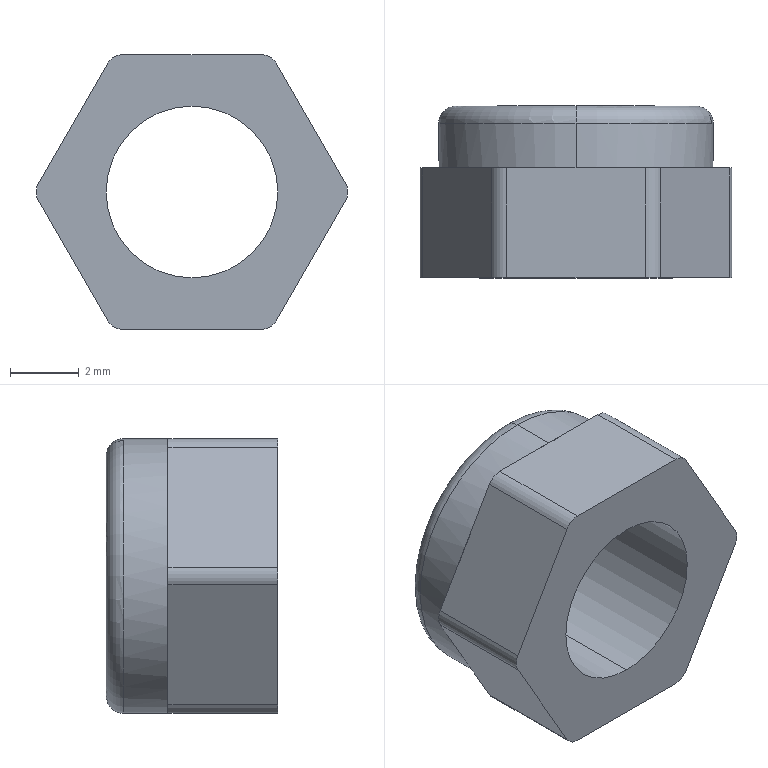Part | SolidWorks | features Extrusion 1, Fillet 1, ICE 1 | 1 solid | 28 faces | box 9.083 x 5 x 8 mm | volume 167.216 mm3 | plane 14 | cylinder 10 | torus 4 | commonest cylinder face diameters 1 x6 5 x2 8 x2
STEP:
#1=CARTESIAN_POINT('',(0.,4.5,-4.));
#2=VERTEX_POINT('',#1);
#3=CARTESIAN_POINT('',(0.,4.5,4.));
#4=VERTEX_POINT('',#3);
#5=CARTESIAN_POINT('',(0.,4.5,0.));
#6=DIRECTION('',(0.,-1.,0.));
#7=DIRECTION('',(0.,0.,1.));
#8=AXIS2_PLACEMENT_3D('',#5,#6,#7);
#9=CIRCLE('',#8,4.);
#10=EDGE_CURVE('',#2,#4,#9,.T.);
#11=ORIENTED_EDGE('',*,*,#10,.F.);
#12=CARTESIAN_POINT('',(0.,5.,-3.5));
#13=VERTEX_POINT('',#12);
#14=CARTESIAN_POINT('',(0.,4.5,-3.5));
#15=DIRECTION('',(1.,0.,0.));
#16=DIRECTION('',(0.,0.,-1.));
#17=AXIS2_PLACEMENT_3D('',#14,#15,#16);
#18=CIRCLE('',#17,0.5);
#19=EDGE_CURVE('',#2,#13,#18,.T.);
#20=ORIENTED_EDGE('',*,*,#19,.T.);
#21=CARTESIAN_POINT('',(0.,5.,3.5));
#22=VERTEX_POINT('',#21);
#23=CARTESIAN_POINT('',(0.,5.,0.));
#24=DIRECTION('',(0.,1.,0.));
#25=DIRECTION('',(0.,0.,1.));
#26=AXIS2_PLACEMENT_3D('',#23,#24,#25);
#27=CIRCLE('',#26,3.5);
#28=EDGE_CURVE('',#22,#13,#27,.T.);
#29=ORIENTED_EDGE('',*,*,#28,.F.);
#30=CARTESIAN_POINT('',(0.,4.5,3.5));
#31=DIRECTION('',(-1.,0.,0.));
#32=DIRECTION('',(0.,0.,1.));
#33=AXIS2_PLACEMENT_3D('',#30,#31,#32);
#34=CIRCLE('',#33,0.5);
#35=EDGE_CURVE('',#4,#22,#34,.T.);
#36=ORIENTED_EDGE('',*,*,#35,.F.);
#37=EDGE_LOOP('',(#11,#20,#29,#36));
#38=FACE_OUTER_BOUND('',#37,.T.);
#39=CARTESIAN_POINT('',(0.,4.5,0.));
#40=DIRECTION('',(0.,1.,0.));
#41=DIRECTION('',(0.,0.,1.));
#42=AXIS2_PLACEMENT_3D('',#39,#40,#41);
#43=TOROIDAL_SURFACE('',#42,3.5,0.5);
#44=ADVANCED_FACE('',(#38),#43,.T.);
#45=CARTESIAN_POINT('',(0.,5.,-3.));
#46=VERTEX_POINT('',#45);
#47=CARTESIAN_POINT('',(0.,5.,3.));
#48=VERTEX_POINT('',#47);
#49=CARTESIAN_POINT('',(0.,5.,0.));
#50=DIRECTION('',(0.,-1.,0.));
#51=DIRECTION('',(0.,0.,1.));
#52=AXIS2_PLACEMENT_3D('',#49,#50,#51);
#53=CIRCLE('',#52,3.);
#54=EDGE_CURVE('',#46,#48,#53,.T.);
#55=ORIENTED_EDGE('',*,*,#54,.F.);
#56=CARTESIAN_POINT('',(0.,4.5,-2.5));
#57=VERTEX_POINT('',#56);
#58=CARTESIAN_POINT('',(0.,4.5,-3.));
#59=DIRECTION('',(1.,0.,0.));
#60=DIRECTION('',(0.,0.,-1.));
#61=AXIS2_PLACEMENT_3D('',#58,#59,#60);
#62=CIRCLE('',#61,0.5);
#63=EDGE_CURVE('',#46,#57,#62,.T.);
#64=ORIENTED_EDGE('',*,*,#63,.T.);
#65=CARTESIAN_POINT('',(0.,4.5,2.5));
#66=VERTEX_POINT('',#65);
#67=CARTESIAN_POINT('',(0.,4.5,0.));
#68=DIRECTION('',(0.,1.,0.));
#69=DIRECTION('',(0.,0.,1.));
#70=AXIS2_PLACEMENT_3D('',#67,#68,#69);
#71=CIRCLE('',#70,2.5);
#72=EDGE_CURVE('',#66,#57,#71,.T.);
#73=ORIENTED_EDGE('',*,*,#72,.F.);
#74=CARTESIAN_POINT('',(0.,4.5,3.));
#75=DIRECTION('',(-1.,0.,0.));
#76=DIRECTION('',(0.,0.,1.));
#77=AXIS2_PLACEMENT_3D('',#74,#75,#76);
#78=CIRCLE('',#77,0.5);
#79=EDGE_CURVE('',#48,#66,#78,.T.);
#80=ORIENTED_EDGE('',*,*,#79,.F.);
#81=EDGE_LOOP('',(#55,#64,#73,#80));
#82=FACE_OUTER_BOUND('',#81,.T.);
#83=CARTESIAN_POINT('',(0.,4.5,0.));
#84=DIRECTION('',(0.,1.,0.));
#85=DIRECTION('',(0.,0.,1.));
#86=AXIS2_PLACEMENT_3D('',#83,#84,#85);
#87=TOROIDAL_SURFACE('',#86,3.,0.5);
#88=ADVANCED_FACE('',(#82),#87,.T.);
#89=ORIENTED_EDGE('',*,*,#10,.T.);
#90=CARTESIAN_POINT('',(0.,3.2,4.));
#91=VERTEX_POINT('',#90);
#92=CARTESIAN_POINT('',(0.,5.,4.));
#93=DIRECTION('',(0.,-1.,0.));
#94=VECTOR('',#93,1000.);
#95=LINE('',#92,#94);
#96=EDGE_CURVE('',#4,#91,#95,.T.);
#97=ORIENTED_EDGE('',*,*,#96,.T.);
#98=CARTESIAN_POINT('',(3.464,3.2,2.));
#99=VERTEX_POINT('',#98);
#100=CARTESIAN_POINT('',(0.,3.2,0.));
#101=DIRECTION('',(0.,1.,0.));
#102=DIRECTION('',(0.,0.,1.));
#103=AXIS2_PLACEMENT_3D('',#100,#101,#102);
#104=CIRCLE('',#103,4.);
#105=EDGE_CURVE('',#91,#99,#104,.T.);
#106=ORIENTED_EDGE('',*,*,#105,.T.);
#107=CARTESIAN_POINT('',(3.464,3.2,-2.));
#108=VERTEX_POINT('',#107);
#109=CARTESIAN_POINT('',(0.,3.2,0.));
#110=DIRECTION('',(0.,1.,0.));
#111=DIRECTION('',(0.,0.,1.));
#112=AXIS2_PLACEMENT_3D('',#109,#110,#111);
#113=CIRCLE('',#112,4.);
#114=EDGE_CURVE('',#99,#108,#113,.T.);
#115=ORIENTED_EDGE('',*,*,#114,.T.);
#116=CARTESIAN_POINT('',(0.,3.2,-4.));
#117=VERTEX_POINT('',#116);
#118=CARTESIAN_POINT('',(0.,3.2,0.));
#119=DIRECTION('',(0.,1.,0.));
#120=DIRECTION('',(0.,0.,1.));
#121=AXIS2_PLACEMENT_3D('',#118,#119,#120);
#122=CIRCLE('',#121,4.);
#123=EDGE_CURVE('',#108,#117,#122,.T.);
#124=ORIENTED_EDGE('',*,*,#123,.T.);
#125=CARTESIAN_POINT('',(0.,5.,-4.));
#126=DIRECTION('',(0.,-1.,0.));
#127=VECTOR('',#126,1000.);
#128=LINE('',#125,#127);
#129=EDGE_CURVE('',#2,#117,#128,.T.);
#130=ORIENTED_EDGE('',*,*,#129,.F.);
#131=EDGE_LOOP('',(#89,#97,#106,#115,#124,#130));
#132=FACE_OUTER_BOUND('',#131,.T.);
#133=CARTESIAN_POINT('',(0.,5.,0.));
#134=DIRECTION('',(0.,-1.,0.));
#135=DIRECTION('',(0.,0.,-1.));
#136=AXIS2_PLACEMENT_3D('',#133,#134,#135);
#137=CYLINDRICAL_SURFACE('',#136,4.);
#138=ADVANCED_FACE('',(#132),#137,.T.);
#139=CARTESIAN_POINT('',(0.,4.5,0.));
#140=DIRECTION('',(0.,1.,0.));
#141=DIRECTION('',(0.,0.,1.));
#142=AXIS2_PLACEMENT_3D('',#139,#140,#141);
#143=CIRCLE('',#142,2.5);
#144=EDGE_CURVE('',#57,#66,#143,.T.);
#145=ORIENTED_EDGE('',*,*,#144,.T.);
#146=CARTESIAN_POINT('',(0.,0.,2.5));
#147=VERTEX_POINT('',#146);
#148=CARTESIAN_POINT('',(0.,3.2,2.5));
#149=DIRECTION('',(0.,-1.,0.));
#150=VECTOR('',#149,1000.);
#151=LINE('',#148,#150);
#152=EDGE_CURVE('',#66,#147,#151,.T.);
#153=ORIENTED_EDGE('',*,*,#152,.T.);
#154=CARTESIAN_POINT('',(0.,0.,-2.5));
#155=VERTEX_POINT('',#154);
#156=CARTESIAN_POINT('',(0.,0.,0.));
#157=DIRECTION('',(0.,1.,0.));
#158=DIRECTION('',(0.,0.,1.));
#159=AXIS2_PLACEMENT_3D('',#156,#157,#158);
#160=CIRCLE('',#159,2.5);
#161=EDGE_CURVE('',#155,#147,#160,.T.);
#162=ORIENTED_EDGE('',*,*,#161,.F.);
#163=CARTESIAN_POINT('',(0.,3.2,-2.5));
#164=DIRECTION('',(0.,-1.,0.));
#165=VECTOR('',#164,1000.);
#166=LINE('',#163,#165);
#167=EDGE_CURVE('',#57,#155,#166,.T.);
#168=ORIENTED_EDGE('',*,*,#167,.F.);
#169=EDGE_LOOP('',(#145,#153,#162,#168));
#170=FACE_OUTER_BOUND('',#169,.T.);
#171=CARTESIAN_POINT('',(0.,3.2,0.));
#172=DIRECTION('',(0.,-1.,0.));
#173=DIRECTION('',(0.,0.,-1.));
#174=AXIS2_PLACEMENT_3D('',#171,#172,#173);
#175=CYLINDRICAL_SURFACE('',#174,2.5);
#176=ADVANCED_FACE('',(#170),#175,.F.);
#177=CARTESIAN_POINT('',(2.021,3.2,4.));
#178=VERTEX_POINT('',#177);
#179=CARTESIAN_POINT('',(-2.309,3.2,4.));
#180=DIRECTION('',(1.,0.,0.));
#181=VECTOR('',#180,1000.);
#182=LINE('',#179,#181);
#183=EDGE_CURVE('',#91,#178,#182,.T.);
#184=ORIENTED_EDGE('',*,*,#183,.T.);
#185=CARTESIAN_POINT('',(2.454,3.2,3.75));
#186=VERTEX_POINT('',#185);
#187=CARTESIAN_POINT('',(2.021,3.2,3.5));
#188=DIRECTION('',(0.,1.,0.));
#189=DIRECTION('',(0.,0.,1.));
#190=AXIS2_PLACEMENT_3D('',#187,#188,#189);
#191=CIRCLE('',#190,0.5);
#192=EDGE_CURVE('',#178,#186,#191,.T.);
#193=ORIENTED_EDGE('',*,*,#192,.T.);
#194=CARTESIAN_POINT('',(2.309,3.2,4.));
#195=DIRECTION('',(0.5,0.,-0.866));
#196=VECTOR('',#195,1000.);
#197=LINE('',#194,#196);
#198=EDGE_CURVE('',#186,#99,#197,.T.);
#199=ORIENTED_EDGE('',*,*,#198,.T.);
#200=ORIENTED_EDGE('',*,*,#105,.F.);
#201=EDGE_LOOP('',(#184,#193,#199,#200));
#202=FACE_OUTER_BOUND('',#201,.T.);
#203=CARTESIAN_POINT('',(0.,3.2,0.));
#204=DIRECTION('',(0.,1.,0.));
#205=DIRECTION('',(0.,0.,1.));
#206=AXIS2_PLACEMENT_3D('',#203,#204,#205);
#207=PLANE('',#206);
#208=ADVANCED_FACE('',(#202),#207,.T.);
#209=CARTESIAN_POINT('',(4.474,3.2,0.25));
#210=VERTEX_POINT('',#209);
#211=CARTESIAN_POINT('',(2.309,3.2,4.));
#212=DIRECTION('',(0.5,0.,-0.866));
#213=VECTOR('',#212,1000.);
#214=LINE('',#211,#213);
#215=EDGE_CURVE('',#99,#210,#214,.T.);
#216=ORIENTED_EDGE('',*,*,#215,.T.);
#217=CARTESIAN_POINT('',(4.474,3.2,-0.25));
#218=VERTEX_POINT('',#217);
#219=CARTESIAN_POINT('',(4.041,3.2,0.));
#220=DIRECTION('',(0.,1.,0.));
#221=DIRECTION('',(0.,0.,1.));
#222=AXIS2_PLACEMENT_3D('',#219,#220,#221);
#223=CIRCLE('',#222,0.5);
#224=EDGE_CURVE('',#210,#218,#223,.T.);
#225=ORIENTED_EDGE('',*,*,#224,.T.);
#226=CARTESIAN_POINT('',(4.619,3.2,0.));
#227=DIRECTION('',(-0.5,0.,-0.866));
#228=VECTOR('',#227,1000.);
#229=LINE('',#226,#228);
#230=EDGE_CURVE('',#218,#108,#229,.T.);
#231=ORIENTED_EDGE('',*,*,#230,.T.);
#232=ORIENTED_EDGE('',*,*,#114,.F.);
#233=EDGE_LOOP('',(#216,#225,#231,#232));
#234=FACE_OUTER_BOUND('',#233,.T.);
#235=CARTESIAN_POINT('',(0.,3.2,0.));
#236=DIRECTION('',(0.,1.,0.));
#237=DIRECTION('',(0.,0.,1.));
#238=AXIS2_PLACEMENT_3D('',#235,#236,#237);
#239=PLANE('',#238);
#240=ADVANCED_FACE('',(#234),#239,.T.);
#241=CARTESIAN_POINT('',(2.454,3.2,-3.75));
#242=VERTEX_POINT('',#241);
#243=CARTESIAN_POINT('',(4.619,3.2,0.));
#244=DIRECTION('',(-0.5,0.,-0.866));
#245=VECTOR('',#244,1000.);
#246=LINE('',#243,#245);
#247=EDGE_CURVE('',#108,#242,#246,.T.);
#248=ORIENTED_EDGE('',*,*,#247,.T.);
#249=CARTESIAN_POINT('',(2.021,3.2,-4.));
#250=VERTEX_POINT('',#249);
#251=CARTESIAN_POINT('',(2.021,3.2,-3.5));
#252=DIRECTION('',(0.,1.,0.));
#253=DIRECTION('',(0.,0.,1.));
#254=AXIS2_PLACEMENT_3D('',#251,#252,#253);
#255=CIRCLE('',#254,0.5);
#256=EDGE_CURVE('',#242,#250,#255,.T.);
#257=ORIENTED_EDGE('',*,*,#256,.T.);
#258=CARTESIAN_POINT('',(2.309,3.2,-4.));
#259=DIRECTION('',(-1.,0.,0.));
#260=VECTOR('',#259,1000.);
#261=LINE('',#258,#260);
#262=EDGE_CURVE('',#250,#117,#261,.T.);
#263=ORIENTED_EDGE('',*,*,#262,.T.);
#264=ORIENTED_EDGE('',*,*,#123,.F.);
#265=EDGE_LOOP('',(#248,#257,#263,#264));
#266=FACE_OUTER_BOUND('',#265,.T.);
#267=CARTESIAN_POINT('',(0.,3.2,0.));
#268=DIRECTION('',(0.,1.,0.));
#269=DIRECTION('',(0.,0.,1.));
#270=AXIS2_PLACEMENT_3D('',#267,#268,#269);
#271=PLANE('',#270);
#272=ADVANCED_FACE('',(#266),#271,.T.);
#273=CARTESIAN_POINT('',(-2.021,3.2,-4.));
#274=VERTEX_POINT('',#273);
#275=CARTESIAN_POINT('',(2.309,3.2,-4.));
#276=DIRECTION('',(-1.,0.,0.));
#277=VECTOR('',#276,1000.);
#278=LINE('',#275,#277);
#279=EDGE_CURVE('',#117,#274,#278,.T.);
#280=ORIENTED_EDGE('',*,*,#279,.T.);
#281=CARTESIAN_POINT('',(-2.454,3.2,-3.75));
#282=VERTEX_POINT('',#281);
#283=CARTESIAN_POINT('',(-2.021,3.2,-3.5));
#284=DIRECTION('',(0.,1.,0.));
#285=DIRECTION('',(0.,0.,1.));
#286=AXIS2_PLACEMENT_3D('',#283,#284,#285);
#287=CIRCLE('',#286,0.5);
#288=EDGE_CURVE('',#274,#282,#287,.T.);
#289=ORIENTED_EDGE('',*,*,#288,.T.);
#290=CARTESIAN_POINT('',(-3.464,3.2,-2.));
#291=VERTEX_POINT('',#290);
#292=CARTESIAN_POINT('',(-2.309,3.2,-4.));
#293=DIRECTION('',(-0.5,0.,0.866));
#294=VECTOR('',#293,1000.);
#295=LINE('',#292,#294);
#296=EDGE_CURVE('',#282,#291,#295,.T.);
#297=ORIENTED_EDGE('',*,*,#296,.T.);
#298=CARTESIAN_POINT('',(0.,3.2,0.));
#299=DIRECTION('',(0.,1.,0.));
#300=DIRECTION('',(0.,0.,1.));
#301=AXIS2_PLACEMENT_3D('',#298,#299,#300);
#302=CIRCLE('',#301,4.);
#303=EDGE_CURVE('',#117,#291,#302,.T.);
#304=ORIENTED_EDGE('',*,*,#303,.F.);
#305=EDGE_LOOP('',(#280,#289,#297,#304));
#306=FACE_OUTER_BOUND('',#305,.T.);
#307=CARTESIAN_POINT('',(0.,3.2,0.));
#308=DIRECTION('',(0.,1.,0.));
#309=DIRECTION('',(0.,0.,1.));
#310=AXIS2_PLACEMENT_3D('',#307,#308,#309);
#311=PLANE('',#310);
#312=ADVANCED_FACE('',(#306),#311,.T.);
#313=CARTESIAN_POINT('',(-4.474,3.2,-0.25));
#314=VERTEX_POINT('',#313);
#315=CARTESIAN_POINT('',(-2.309,3.2,-4.));
#316=DIRECTION('',(-0.5,0.,0.866));
#317=VECTOR('',#316,1000.);
#318=LINE('',#315,#317);
#319=EDGE_CURVE('',#291,#314,#318,.T.);
#320=ORIENTED_EDGE('',*,*,#319,.T.);
#321=CARTESIAN_POINT('',(-4.474,3.2,0.25));
#322=VERTEX_POINT('',#321);
#323=CARTESIAN_POINT('',(-4.041,3.2,0.));
#324=DIRECTION('',(0.,1.,0.));
#325=DIRECTION('',(0.,0.,1.));
#326=AXIS2_PLACEMENT_3D('',#323,#324,#325);
#327=CIRCLE('',#326,0.5);
#328=EDGE_CURVE('',#314,#322,#327,.T.);
#329=ORIENTED_EDGE('',*,*,#328,.T.);
#330=CARTESIAN_POINT('',(-3.464,3.2,2.));
#331=VERTEX_POINT('',#330);
#332=CARTESIAN_POINT('',(-4.619,3.2,0.));
#333=DIRECTION('',(0.5,0.,0.866));
#334=VECTOR('',#333,1000.);
#335=LINE('',#332,#334);
#336=EDGE_CURVE('',#322,#331,#335,.T.);
#337=ORIENTED_EDGE('',*,*,#336,.T.);
#338=CARTESIAN_POINT('',(0.,3.2,0.));
#339=DIRECTION('',(0.,1.,0.));
#340=DIRECTION('',(0.,0.,1.));
#341=AXIS2_PLACEMENT_3D('',#338,#339,#340);
#342=CIRCLE('',#341,4.);
#343=EDGE_CURVE('',#291,#331,#342,.T.);
#344=ORIENTED_EDGE('',*,*,#343,.F.);
#345=EDGE_LOOP('',(#320,#329,#337,#344));
#346=FACE_OUTER_BOUND('',#345,.T.);
#347=CARTESIAN_POINT('',(0.,3.2,0.));
#348=DIRECTION('',(0.,1.,0.));
#349=DIRECTION('',(0.,0.,1.));
#350=AXIS2_PLACEMENT_3D('',#347,#348,#349);
#351=PLANE('',#350);
#352=ADVANCED_FACE('',(#346),#351,.T.);
#353=CARTESIAN_POINT('',(-2.454,3.2,3.75));
#354=VERTEX_POINT('',#353);
#355=CARTESIAN_POINT('',(-4.619,3.2,0.));
#356=DIRECTION('',(0.5,0.,0.866));
#357=VECTOR('',#356,1000.);
#358=LINE('',#355,#357);
#359=EDGE_CURVE('',#331,#354,#358,.T.);
#360=ORIENTED_EDGE('',*,*,#359,.T.);
#361=CARTESIAN_POINT('',(-2.021,3.2,4.));
#362=VERTEX_POINT('',#361);
#363=CARTESIAN_POINT('',(-2.021,3.2,3.5));
#364=DIRECTION('',(0.,1.,0.));
#365=DIRECTION('',(0.,0.,1.));
#366=AXIS2_PLACEMENT_3D('',#363,#364,#365);
#367=CIRCLE('',#366,0.5);
#368=EDGE_CURVE('',#354,#362,#367,.T.);
#369=ORIENTED_EDGE('',*,*,#368,.T.);
#370=CARTESIAN_POINT('',(-2.309,3.2,4.));
#371=DIRECTION('',(1.,0.,0.));
#372=VECTOR('',#371,1000.);
#373=LINE('',#370,#372);
#374=EDGE_CURVE('',#362,#91,#373,.T.);
#375=ORIENTED_EDGE('',*,*,#374,.T.);
#376=CARTESIAN_POINT('',(0.,3.2,0.));
#377=DIRECTION('',(0.,1.,0.));
#378=DIRECTION('',(0.,0.,1.));
#379=AXIS2_PLACEMENT_3D('',#376,#377,#378);
#380=CIRCLE('',#379,4.);
#381=EDGE_CURVE('',#331,#91,#380,.T.);
#382=ORIENTED_EDGE('',*,*,#381,.F.);
#383=EDGE_LOOP('',(#360,#369,#375,#382));
#384=FACE_OUTER_BOUND('',#383,.T.);
#385=CARTESIAN_POINT('',(0.,3.2,0.));
#386=DIRECTION('',(0.,1.,0.));
#387=DIRECTION('',(0.,0.,1.));
#388=AXIS2_PLACEMENT_3D('',#385,#386,#387);
#389=PLANE('',#388);
#390=ADVANCED_FACE('',(#384),#389,.T.);
#391=CARTESIAN_POINT('',(-4.474,0.,0.25));
#392=VERTEX_POINT('',#391);
#393=CARTESIAN_POINT('',(-2.454,0.,3.75));
#394=VERTEX_POINT('',#393);
#395=CARTESIAN_POINT('',(-4.619,0.,0.));
#396=DIRECTION('',(0.5,0.,0.866));
#397=VECTOR('',#396,1000.);
#398=LINE('',#395,#397);
#399=EDGE_CURVE('',#392,#394,#398,.T.);
#400=ORIENTED_EDGE('',*,*,#399,.F.);
#401=CARTESIAN_POINT('',(-4.474,0.,-0.25));
#402=VERTEX_POINT('',#401);
#403=CARTESIAN_POINT('',(-4.041,0.,0.));
#404=DIRECTION('',(0.,-1.,0.));
#405=DIRECTION('',(0.,0.,1.));
#406=AXIS2_PLACEMENT_3D('',#403,#404,#405);
#407=CIRCLE('',#406,0.5);
#408=EDGE_CURVE('',#392,#402,#407,.T.);
#409=ORIENTED_EDGE('',*,*,#408,.T.);
#410=CARTESIAN_POINT('',(-2.454,0.,-3.75));
#411=VERTEX_POINT('',#410);
#412=CARTESIAN_POINT('',(-2.309,0.,-4.));
#413=DIRECTION('',(-0.5,0.,0.866));
#414=VECTOR('',#413,1000.);
#415=LINE('',#412,#414);
#416=EDGE_CURVE('',#411,#402,#415,.T.);
#417=ORIENTED_EDGE('',*,*,#416,.F.);
#418=CARTESIAN_POINT('',(-2.021,0.,-4.));
#419=VERTEX_POINT('',#418);
#420=CARTESIAN_POINT('',(-2.021,0.,-3.5));
#421=DIRECTION('',(0.,-1.,0.));
#422=DIRECTION('',(0.,0.,1.));
#423=AXIS2_PLACEMENT_3D('',#420,#421,#422);
#424=CIRCLE('',#423,0.5);
#425=EDGE_CURVE('',#411,#419,#424,.T.);
#426=ORIENTED_EDGE('',*,*,#425,.T.);
#427=CARTESIAN_POINT('',(2.021,0.,-4.));
#428=VERTEX_POINT('',#427);
#429=CARTESIAN_POINT('',(2.309,0.,-4.));
#430=DIRECTION('',(-1.,0.,0.));
#431=VECTOR('',#430,1000.);
#432=LINE('',#429,#431);
#433=EDGE_CURVE('',#428,#419,#432,.T.);
#434=ORIENTED_EDGE('',*,*,#433,.F.);
#435=CARTESIAN_POINT('',(2.454,0.,-3.75));
#436=VERTEX_POINT('',#435);
#437=CARTESIAN_POINT('',(2.021,0.,-3.5));
#438=DIRECTION('',(0.,-1.,0.));
#439=DIRECTION('',(0.,0.,1.));
#440=AXIS2_PLACEMENT_3D('',#437,#438,#439);
#441=CIRCLE('',#440,0.5);
#442=EDGE_CURVE('',#428,#436,#441,.T.);
#443=ORIENTED_EDGE('',*,*,#442,.T.);
#444=CARTESIAN_POINT('',(4.474,0.,-0.25));
#445=VERTEX_POINT('',#444);
#446=CARTESIAN_POINT('',(4.619,0.,0.));
#447=DIRECTION('',(-0.5,0.,-0.866));
#448=VECTOR('',#447,1000.);
#449=LINE('',#446,#448);
#450=EDGE_CURVE('',#445,#436,#449,.T.);
#451=ORIENTED_EDGE('',*,*,#450,.F.);
#452=CARTESIAN_POINT('',(4.474,0.,0.25));
#453=VERTEX_POINT('',#452);
#454=CARTESIAN_POINT('',(4.041,0.,0.));
#455=DIRECTION('',(0.,-1.,0.));
#456=DIRECTION('',(0.,0.,1.));
#457=AXIS2_PLACEMENT_3D('',#454,#455,#456);
#458=CIRCLE('',#457,0.5);
#459=EDGE_CURVE('',#445,#453,#458,.T.);
#460=ORIENTED_EDGE('',*,*,#459,.T.);
#461=CARTESIAN_POINT('',(2.454,0.,3.75));
#462=VERTEX_POINT('',#461);
#463=CARTESIAN_POINT('',(2.309,0.,4.));
#464=DIRECTION('',(0.5,0.,-0.866));
#465=VECTOR('',#464,1000.);
#466=LINE('',#463,#465);
#467=EDGE_CURVE('',#462,#453,#466,.T.);
#468=ORIENTED_EDGE('',*,*,#467,.F.);
#469=CARTESIAN_POINT('',(2.021,0.,4.));
#470=VERTEX_POINT('',#469);
#471=CARTESIAN_POINT('',(2.021,0.,3.5));
#472=DIRECTION('',(0.,-1.,0.));
#473=DIRECTION('',(0.,0.,1.));
#474=AXIS2_PLACEMENT_3D('',#471,#472,#473);
#475=CIRCLE('',#474,0.5);
#476=EDGE_CURVE('',#462,#470,#475,.T.);
#477=ORIENTED_EDGE('',*,*,#476,.T.);
#478=CARTESIAN_POINT('',(-2.021,0.,4.));
#479=VERTEX_POINT('',#478);
#480=CARTESIAN_POINT('',(-2.309,0.,4.));
#481=DIRECTION('',(1.,0.,0.));
#482=VECTOR('',#481,1000.);
#483=LINE('',#480,#482);
#484=EDGE_CURVE('',#479,#470,#483,.T.);
#485=ORIENTED_EDGE('',*,*,#484,.F.);
#486=CARTESIAN_POINT('',(-2.021,0.,3.5));
#487=DIRECTION('',(0.,-1.,0.));
#488=DIRECTION('',(0.,0.,1.));
#489=AXIS2_PLACEMENT_3D('',#486,#487,#488);
#490=CIRCLE('',#489,0.5);
#491=EDGE_CURVE('',#479,#394,#490,.T.);
#492=ORIENTED_EDGE('',*,*,#491,.T.);
#493=EDGE_LOOP('',(#400,#409,#417,#426,#434,#443,#451,#460,#468,#477,#485,#492));
#494=FACE_OUTER_BOUND('',#493,.T.);
#495=ORIENTED_EDGE('',*,*,#161,.T.);
#496=CARTESIAN_POINT('',(0.,0.,0.));
#497=DIRECTION('',(0.,1.,0.));
#498=DIRECTION('',(0.,0.,1.));
#499=AXIS2_PLACEMENT_3D('',#496,#497,#498);
#500=CIRCLE('',#499,2.5);
#501=EDGE_CURVE('',#147,#155,#500,.T.);
#502=ORIENTED_EDGE('',*,*,#501,.T.);
#503=EDGE_LOOP('',(#495,#502));
#504=FACE_BOUND('',#503,.T.);
#505=CARTESIAN_POINT('',(0.,0.,0.));
#506=DIRECTION('',(0.,1.,0.));
#507=DIRECTION('',(0.,0.,1.));
#508=AXIS2_PLACEMENT_3D('',#505,#506,#507);
#509=PLANE('',#508);
#510=ADVANCED_FACE('',(#494,#504),#509,.F.);
#511=ORIENTED_EDGE('',*,*,#467,.T.);
#512=CARTESIAN_POINT('',(4.474,3.2,0.25));
#513=DIRECTION('',(0.,1.,0.));
#514=VECTOR('',#513,1000.);
#515=LINE('',#512,#514);
#516=EDGE_CURVE('',#453,#210,#515,.T.);
#517=ORIENTED_EDGE('',*,*,#516,.T.);
#518=ORIENTED_EDGE('',*,*,#215,.F.);
#519=ORIENTED_EDGE('',*,*,#198,.F.);
#520=CARTESIAN_POINT('',(2.454,3.2,3.75));
#521=DIRECTION('',(0.,-1.,0.));
#522=VECTOR('',#521,1000.);
#523=LINE('',#520,#522);
#524=EDGE_CURVE('',#186,#462,#523,.T.);
#525=ORIENTED_EDGE('',*,*,#524,.T.);
#526=EDGE_LOOP('',(#511,#517,#518,#519,#525));
#527=FACE_OUTER_BOUND('',#526,.T.);
#528=CARTESIAN_POINT('',(2.309,3.2,4.));
#529=DIRECTION('',(-0.866,0.,-0.5));
#530=DIRECTION('',(-0.5,0.,0.866));
#531=AXIS2_PLACEMENT_3D('',#528,#529,#530);
#532=PLANE('',#531);
#533=ADVANCED_FACE('',(#527),#532,.F.);
#534=ORIENTED_EDGE('',*,*,#450,.T.);
#535=CARTESIAN_POINT('',(2.454,3.2,-3.75));
#536=DIRECTION('',(0.,1.,0.));
#537=VECTOR('',#536,1000.);
#538=LINE('',#535,#537);
#539=EDGE_CURVE('',#436,#242,#538,.T.);
#540=ORIENTED_EDGE('',*,*,#539,.T.);
#541=ORIENTED_EDGE('',*,*,#247,.F.);
#542=ORIENTED_EDGE('',*,*,#230,.F.);
#543=CARTESIAN_POINT('',(4.474,3.2,-0.25));
#544=DIRECTION('',(0.,-1.,0.));
#545=VECTOR('',#544,1000.);
#546=LINE('',#543,#545);
#547=EDGE_CURVE('',#218,#445,#546,.T.);
#548=ORIENTED_EDGE('',*,*,#547,.T.);
#549=EDGE_LOOP('',(#534,#540,#541,#542,#548));
#550=FACE_OUTER_BOUND('',#549,.T.);
#551=CARTESIAN_POINT('',(4.619,3.2,0.));
#552=DIRECTION('',(-0.866,0.,0.5));
#553=DIRECTION('',(0.5,0.,0.866));
#554=AXIS2_PLACEMENT_3D('',#551,#552,#553);
#555=PLANE('',#554);
#556=ADVANCED_FACE('',(#550),#555,.F.);
#557=ORIENTED_EDGE('',*,*,#433,.T.);
#558=CARTESIAN_POINT('',(-2.021,3.2,-4.));
#559=DIRECTION('',(0.,1.,0.));
#560=VECTOR('',#559,1000.);
#561=LINE('',#558,#560);
#562=EDGE_CURVE('',#419,#274,#561,.T.);
#563=ORIENTED_EDGE('',*,*,#562,.T.);
#564=ORIENTED_EDGE('',*,*,#279,.F.);
#565=ORIENTED_EDGE('',*,*,#262,.F.);
#566=CARTESIAN_POINT('',(2.021,3.2,-4.));
#567=DIRECTION('',(0.,-1.,0.));
#568=VECTOR('',#567,1000.);
#569=LINE('',#566,#568);
#570=EDGE_CURVE('',#250,#428,#569,.T.);
#571=ORIENTED_EDGE('',*,*,#570,.T.);
#572=EDGE_LOOP('',(#557,#563,#564,#565,#571));
#573=FACE_OUTER_BOUND('',#572,.T.);
#574=CARTESIAN_POINT('',(2.309,3.2,-4.));
#575=DIRECTION('',(0.,0.,1.));
#576=DIRECTION('',(1.,0.,0.));
#577=AXIS2_PLACEMENT_3D('',#574,#575,#576);
#578=PLANE('',#577);
#579=ADVANCED_FACE('',(#573),#578,.F.);
#580=ORIENTED_EDGE('',*,*,#416,.T.);
#581=CARTESIAN_POINT('',(-4.474,3.2,-0.25));
#582=DIRECTION('',(0.,1.,0.));
#583=VECTOR('',#582,1000.);
#584=LINE('',#581,#583);
#585=EDGE_CURVE('',#402,#314,#584,.T.);
#586=ORIENTED_EDGE('',*,*,#585,.T.);
#587=ORIENTED_EDGE('',*,*,#319,.F.);
#588=ORIENTED_EDGE('',*,*,#296,.F.);
#589=CARTESIAN_POINT('',(-2.454,3.2,-3.75));
#590=DIRECTION('',(0.,-1.,0.));
#591=VECTOR('',#590,1000.);
#592=LINE('',#589,#591);
#593=EDGE_CURVE('',#282,#411,#592,.T.);
#594=ORIENTED_EDGE('',*,*,#593,.T.);
#595=EDGE_LOOP('',(#580,#586,#587,#588,#594));
#596=FACE_OUTER_BOUND('',#595,.T.);
#597=CARTESIAN_POINT('',(-2.309,3.2,-4.));
#598=DIRECTION('',(0.866,0.,0.5));
#599=DIRECTION('',(0.5,0.,-0.866));
#600=AXIS2_PLACEMENT_3D('',#597,#598,#599);
#601=PLANE('',#600);
#602=ADVANCED_FACE('',(#596),#601,.F.);
#603=ORIENTED_EDGE('',*,*,#336,.F.);
#604=CARTESIAN_POINT('',(-4.474,3.2,0.25));
#605=DIRECTION('',(0.,-1.,0.));
#606=VECTOR('',#605,1000.);
#607=LINE('',#604,#606);
#608=EDGE_CURVE('',#322,#392,#607,.T.);
#609=ORIENTED_EDGE('',*,*,#608,.T.);
#610=ORIENTED_EDGE('',*,*,#399,.T.);
#611=CARTESIAN_POINT('',(-2.454,3.2,3.75));
#612=DIRECTION('',(0.,1.,0.));
#613=VECTOR('',#612,1000.);
#614=LINE('',#611,#613);
#615=EDGE_CURVE('',#394,#354,#614,.T.);
#616=ORIENTED_EDGE('',*,*,#615,.T.);
#617=ORIENTED_EDGE('',*,*,#359,.F.);
#618=EDGE_LOOP('',(#603,#609,#610,#616,#617));
#619=FACE_OUTER_BOUND('',#618,.T.);
#620=CARTESIAN_POINT('',(-4.619,3.2,0.));
#621=DIRECTION('',(0.866,0.,-0.5));
#622=DIRECTION('',(-0.5,0.,-0.866));
#623=AXIS2_PLACEMENT_3D('',#620,#621,#622);
#624=PLANE('',#623);
#625=ADVANCED_FACE('',(#619),#624,.F.);
#626=ORIENTED_EDGE('',*,*,#374,.F.);
#627=CARTESIAN_POINT('',(-2.021,3.2,4.));
#628=DIRECTION('',(0.,-1.,0.));
#629=VECTOR('',#628,1000.);
#630=LINE('',#627,#629);
#631=EDGE_CURVE('',#362,#479,#630,.T.);
#632=ORIENTED_EDGE('',*,*,#631,.T.);
#633=ORIENTED_EDGE('',*,*,#484,.T.);
#634=CARTESIAN_POINT('',(2.021,3.2,4.));
#635=DIRECTION('',(0.,1.,0.));
#636=VECTOR('',#635,1000.);
#637=LINE('',#634,#636);
#638=EDGE_CURVE('',#470,#178,#637,.T.);
#639=ORIENTED_EDGE('',*,*,#638,.T.);
#640=ORIENTED_EDGE('',*,*,#183,.F.);
#641=EDGE_LOOP('',(#626,#632,#633,#639,#640));
#642=FACE_OUTER_BOUND('',#641,.T.);
#643=CARTESIAN_POINT('',(-2.309,3.2,4.));
#644=DIRECTION('',(0.,0.,-1.));
#645=DIRECTION('',(-1.,0.,0.));
#646=AXIS2_PLACEMENT_3D('',#643,#644,#645);
#647=PLANE('',#646);
#648=ADVANCED_FACE('',(#642),#647,.F.);
#649=ORIENTED_EDGE('',*,*,#152,.F.);
#650=ORIENTED_EDGE('',*,*,#72,.T.);
#651=ORIENTED_EDGE('',*,*,#167,.T.);
#652=ORIENTED_EDGE('',*,*,#501,.F.);
#653=EDGE_LOOP('',(#649,#650,#651,#652));
#654=FACE_OUTER_BOUND('',#653,.T.);
#655=CARTESIAN_POINT('',(0.,3.2,0.));
#656=DIRECTION('',(0.,-1.,0.));
#657=DIRECTION('',(0.,0.,-1.));
#658=AXIS2_PLACEMENT_3D('',#655,#656,#657);
#659=CYLINDRICAL_SURFACE('',#658,2.5);
#660=ADVANCED_FACE('',(#654),#659,.F.);
#661=CARTESIAN_POINT('',(0.,5.,0.));
#662=DIRECTION('',(0.,-1.,0.));
#663=DIRECTION('',(0.,0.,1.));
#664=AXIS2_PLACEMENT_3D('',#661,#662,#663);
#665=CIRCLE('',#664,3.);
#666=EDGE_CURVE('',#48,#46,#665,.T.);
#667=ORIENTED_EDGE('',*,*,#666,.T.);
#668=ORIENTED_EDGE('',*,*,#54,.T.);
#669=EDGE_LOOP('',(#667,#668));
#670=FACE_BOUND('',#669,.T.);
#671=ORIENTED_EDGE('',*,*,#28,.T.);
#672=CARTESIAN_POINT('',(0.,5.,0.));
#673=DIRECTION('',(0.,1.,0.));
#674=DIRECTION('',(0.,0.,1.));
#675=AXIS2_PLACEMENT_3D('',#672,#673,#674);
#676=CIRCLE('',#675,3.5);
#677=EDGE_CURVE('',#13,#22,#676,.T.);
#678=ORIENTED_EDGE('',*,*,#677,.T.);
#679=EDGE_LOOP('',(#671,#678));
#680=FACE_OUTER_BOUND('',#679,.T.);
#681=CARTESIAN_POINT('',(0.,5.,0.));
#682=DIRECTION('',(0.,1.,0.));
#683=DIRECTION('',(0.,0.,1.));
#684=AXIS2_PLACEMENT_3D('',#681,#682,#683);
#685=PLANE('',#684);
#686=ADVANCED_FACE('',(#670,#680),#685,.T.);
#687=ORIENTED_EDGE('',*,*,#96,.F.);
#688=CARTESIAN_POINT('',(0.,4.5,0.));
#689=DIRECTION('',(0.,-1.,0.));
#690=DIRECTION('',(0.,0.,1.));
#691=AXIS2_PLACEMENT_3D('',#688,#689,#690);
#692=CIRCLE('',#691,4.);
#693=EDGE_CURVE('',#4,#2,#692,.T.);
#694=ORIENTED_EDGE('',*,*,#693,.T.);
#695=ORIENTED_EDGE('',*,*,#129,.T.);
#696=ORIENTED_EDGE('',*,*,#303,.T.);
#697=ORIENTED_EDGE('',*,*,#343,.T.);
#698=ORIENTED_EDGE('',*,*,#381,.T.);
#699=EDGE_LOOP('',(#687,#694,#695,#696,#697,#698));
#700=FACE_OUTER_BOUND('',#699,.T.);
#701=CARTESIAN_POINT('',(0.,5.,0.));
#702=DIRECTION('',(0.,-1.,0.));
#703=DIRECTION('',(0.,0.,-1.));
#704=AXIS2_PLACEMENT_3D('',#701,#702,#703);
#705=CYLINDRICAL_SURFACE('',#704,4.);
#706=ADVANCED_FACE('',(#700),#705,.T.);
#707=ORIENTED_EDGE('',*,*,#63,.F.);
#708=ORIENTED_EDGE('',*,*,#666,.F.);
#709=ORIENTED_EDGE('',*,*,#79,.T.);
#710=ORIENTED_EDGE('',*,*,#144,.F.);
#711=EDGE_LOOP('',(#707,#708,#709,#710));
#712=FACE_OUTER_BOUND('',#711,.T.);
#713=CARTESIAN_POINT('',(0.,4.5,0.));
#714=DIRECTION('',(0.,1.,0.));
#715=DIRECTION('',(0.,0.,1.));
#716=AXIS2_PLACEMENT_3D('',#713,#714,#715);
#717=TOROIDAL_SURFACE('',#716,3.,0.5);
#718=ADVANCED_FACE('',(#712),#717,.T.);
#719=ORIENTED_EDGE('',*,*,#19,.F.);
#720=ORIENTED_EDGE('',*,*,#693,.F.);
#721=ORIENTED_EDGE('',*,*,#35,.T.);
#722=ORIENTED_EDGE('',*,*,#677,.F.);
#723=EDGE_LOOP('',(#719,#720,#721,#722));
#724=FACE_OUTER_BOUND('',#723,.T.);
#725=CARTESIAN_POINT('',(0.,4.5,0.));
#726=DIRECTION('',(0.,1.,0.));
#727=DIRECTION('',(0.,0.,1.));
#728=AXIS2_PLACEMENT_3D('',#725,#726,#727);
#729=TOROIDAL_SURFACE('',#728,3.5,0.5);
#730=ADVANCED_FACE('',(#724),#729,.T.);
#731=ORIENTED_EDGE('',*,*,#328,.F.);
#732=ORIENTED_EDGE('',*,*,#585,.F.);
#733=ORIENTED_EDGE('',*,*,#408,.F.);
#734=ORIENTED_EDGE('',*,*,#608,.F.);
#735=EDGE_LOOP('',(#731,#732,#733,#734));
#736=FACE_OUTER_BOUND('',#735,.T.);
#737=CARTESIAN_POINT('',(-4.041,3.2,0.));
#738=DIRECTION('',(0.,-1.,0.));
#739=DIRECTION('',(0.,0.,-1.));
#740=AXIS2_PLACEMENT_3D('',#737,#738,#739);
#741=CYLINDRICAL_SURFACE('',#740,0.5);
#742=ADVANCED_FACE('',(#736),#741,.T.);
#743=ORIENTED_EDGE('',*,*,#368,.F.);
#744=ORIENTED_EDGE('',*,*,#615,.F.);
#745=ORIENTED_EDGE('',*,*,#491,.F.);
#746=ORIENTED_EDGE('',*,*,#631,.F.);
#747=EDGE_LOOP('',(#743,#744,#745,#746));
#748=FACE_OUTER_BOUND('',#747,.T.);
#749=CARTESIAN_POINT('',(-2.021,3.2,3.5));
#750=DIRECTION('',(0.,-1.,0.));
#751=DIRECTION('',(0.,0.,-1.));
#752=AXIS2_PLACEMENT_3D('',#749,#750,#751);
#753=CYLINDRICAL_SURFACE('',#752,0.5);
#754=ADVANCED_FACE('',(#748),#753,.T.);
#755=ORIENTED_EDGE('',*,*,#288,.F.);
#756=ORIENTED_EDGE('',*,*,#562,.F.);
#757=ORIENTED_EDGE('',*,*,#425,.F.);
#758=ORIENTED_EDGE('',*,*,#593,.F.);
#759=EDGE_LOOP('',(#755,#756,#757,#758));
#760=FACE_OUTER_BOUND('',#759,.T.);
#761=CARTESIAN_POINT('',(-2.021,3.2,-3.5));
#762=DIRECTION('',(0.,-1.,0.));
#763=DIRECTION('',(0.,0.,-1.));
#764=AXIS2_PLACEMENT_3D('',#761,#762,#763);
#765=CYLINDRICAL_SURFACE('',#764,0.5);
#766=ADVANCED_FACE('',(#760),#765,.T.);
#767=ORIENTED_EDGE('',*,*,#256,.F.);
#768=ORIENTED_EDGE('',*,*,#539,.F.);
#769=ORIENTED_EDGE('',*,*,#442,.F.);
#770=ORIENTED_EDGE('',*,*,#570,.F.);
#771=EDGE_LOOP('',(#767,#768,#769,#770));
#772=FACE_OUTER_BOUND('',#771,.T.);
#773=CARTESIAN_POINT('',(2.021,3.2,-3.5));
#774=DIRECTION('',(0.,-1.,0.));
#775=DIRECTION('',(0.,0.,-1.));
#776=AXIS2_PLACEMENT_3D('',#773,#774,#775);
#777=CYLINDRICAL_SURFACE('',#776,0.5);
#778=ADVANCED_FACE('',(#772),#777,.T.);
#779=ORIENTED_EDGE('',*,*,#224,.F.);
#780=ORIENTED_EDGE('',*,*,#516,.F.);
#781=ORIENTED_EDGE('',*,*,#459,.F.);
#782=ORIENTED_EDGE('',*,*,#547,.F.);
#783=EDGE_LOOP('',(#779,#780,#781,#782));
#784=FACE_OUTER_BOUND('',#783,.T.);
#785=CARTESIAN_POINT('',(4.041,3.2,0.));
#786=DIRECTION('',(0.,-1.,0.));
#787=DIRECTION('',(0.,0.,-1.));
#788=AXIS2_PLACEMENT_3D('',#785,#786,#787);
#789=CYLINDRICAL_SURFACE('',#788,0.5);
#790=ADVANCED_FACE('',(#784),#789,.T.);
#791=ORIENTED_EDGE('',*,*,#192,.F.);
#792=ORIENTED_EDGE('',*,*,#638,.F.);
#793=ORIENTED_EDGE('',*,*,#476,.F.);
#794=ORIENTED_EDGE('',*,*,#524,.F.);
#795=EDGE_LOOP('',(#791,#792,#793,#794));
#796=FACE_OUTER_BOUND('',#795,.T.);
#797=CARTESIAN_POINT('',(2.021,3.2,3.5));
#798=DIRECTION('',(0.,-1.,0.));
#799=DIRECTION('',(0.,0.,-1.));
#800=AXIS2_PLACEMENT_3D('',#797,#798,#799);
#801=CYLINDRICAL_SURFACE('',#800,0.5);
#802=ADVANCED_FACE('',(#796),#801,.T.);
#803=CLOSED_SHELL('',(#44,#88,#138,#176,#208,#240,#272,#312,#352,#390,#510,#533,#556,#579,#602,#625,#648,#660,#686,#706,#718,#730,#742,#754,#766,#778,#790,#802));
#804=MANIFOLD_SOLID_BREP('',#803);
#805=CARTESIAN_POINT('',(0.,0.,0.));
#806=DIRECTION('',(0.,0.,1.));
#807=DIRECTION('',(1.,0.,0.));
#808=AXIS2_PLACEMENT_3D('',#805,#806,#807);
#809=(LENGTH_UNIT()NAMED_UNIT(*)SI_UNIT(.MILLI.,.METRE.));
#810=UNCERTAINTY_MEASURE_WITH_UNIT(LENGTH_MEASURE(0.00001),#809,'','');
#811=(NAMED_UNIT(*)PLANE_ANGLE_UNIT()SI_UNIT($,.RADIAN.));
#812=(NAMED_UNIT(*)SI_UNIT($,.STERADIAN.)SOLID_ANGLE_UNIT());
#813=(GEOMETRIC_REPRESENTATION_CONTEXT(3)GLOBAL_UNCERTAINTY_ASSIGNED_CONTEXT((#810))GLOBAL_UNIT_ASSIGNED_CONTEXT((#809,#811,#812))REPRESENTATION_CONTEXT('',''));
#814=ADVANCED_BREP_SHAPE_REPRESENTATION('',(#804,#808),#813);